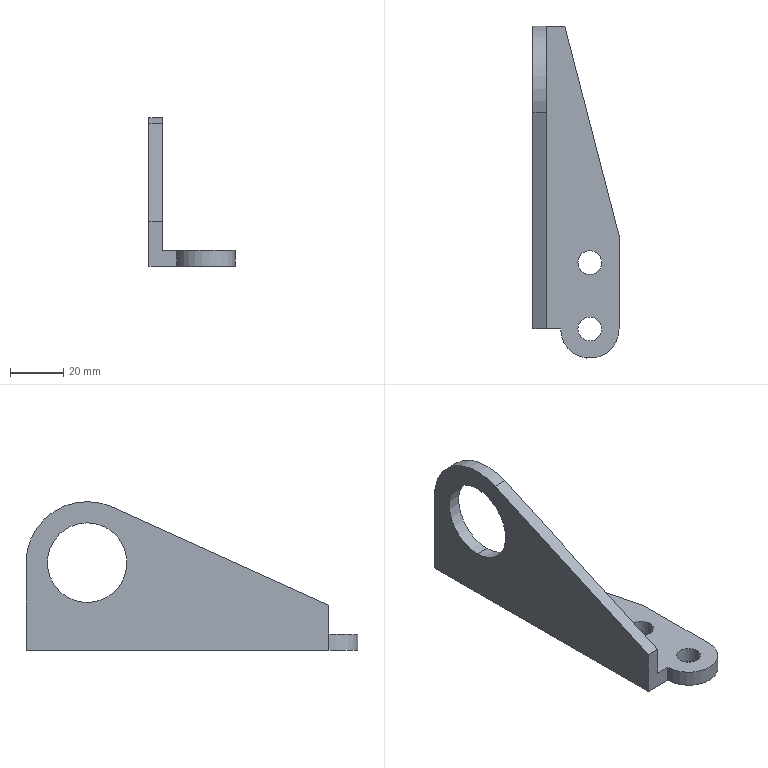Part | SolidWorks | features BaseBody 1 | 1 solid | 17 faces | box 32.409 x 125 x 56 mm | volume 33709 mm3 | plane 9 | cylinder 8 | commonest cylinder face diameters 9 x4 30 x2 22 x1 46 x1
STEP:
#1=CARTESIAN_POINT('',(-12.659,449.35,-210.5));
#2=VERTEX_POINT('',#1);
#3=CARTESIAN_POINT('',(-12.659,449.35,-180.5));
#4=VERTEX_POINT('',#3);
#5=CARTESIAN_POINT('',(-12.659,449.35,-195.5));
#6=DIRECTION('',(-1.,0.,0.));
#7=DIRECTION('',(0.,0.,-1.));
#8=AXIS2_PLACEMENT_3D('',#5,#6,#7);
#9=CIRCLE('',#8,15.);
#10=EDGE_CURVE('',#2,#4,#9,.T.);
#11=ORIENTED_EDGE('',*,*,#10,.T.);
#12=CARTESIAN_POINT('',(-7.659,449.35,-180.5));
#13=VERTEX_POINT('',#12);
#14=CARTESIAN_POINT('',(-12.659,449.35,-180.5));
#15=DIRECTION('',(1.,0.,0.));
#16=VECTOR('',#15,1000.);
#17=LINE('',#14,#16);
#18=EDGE_CURVE('',#4,#13,#17,.T.);
#19=ORIENTED_EDGE('',*,*,#18,.T.);
#20=CARTESIAN_POINT('',(-7.659,449.35,-210.5));
#21=VERTEX_POINT('',#20);
#22=CARTESIAN_POINT('',(-7.659,449.35,-195.5));
#23=DIRECTION('',(-1.,0.,0.));
#24=DIRECTION('',(0.,0.,-1.));
#25=AXIS2_PLACEMENT_3D('',#22,#23,#24);
#26=CIRCLE('',#25,15.);
#27=EDGE_CURVE('',#21,#13,#26,.T.);
#28=ORIENTED_EDGE('',*,*,#27,.F.);
#29=CARTESIAN_POINT('',(-12.659,449.35,-210.5));
#30=DIRECTION('',(1.,0.,0.));
#31=VECTOR('',#30,1000.);
#32=LINE('',#29,#31);
#33=EDGE_CURVE('',#2,#21,#32,.T.);
#34=ORIENTED_EDGE('',*,*,#33,.F.);
#35=EDGE_LOOP('',(#11,#19,#28,#34));
#36=FACE_OUTER_BOUND('',#35,.T.);
#37=CARTESIAN_POINT('',(-12.659,449.35,-195.5));
#38=DIRECTION('',(1.,0.,0.));
#39=DIRECTION('',(0.,0.,-1.));
#40=AXIS2_PLACEMENT_3D('',#37,#38,#39);
#41=CYLINDRICAL_SURFACE('',#40,15.);
#42=ADVANCED_FACE('',(#36),#41,.F.);
#43=CARTESIAN_POINT('',(13.25,358.35,-222.5));
#44=VERTEX_POINT('',#43);
#45=CARTESIAN_POINT('',(4.25,358.35,-222.5));
#46=VERTEX_POINT('',#45);
#47=CARTESIAN_POINT('',(8.75,358.35,-222.5));
#48=DIRECTION('',(0.,0.,-1.));
#49=DIRECTION('',(-1.,0.,0.));
#50=AXIS2_PLACEMENT_3D('',#47,#48,#49);
#51=CIRCLE('',#50,4.5);
#52=EDGE_CURVE('',#44,#46,#51,.T.);
#53=ORIENTED_EDGE('',*,*,#52,.F.);
#54=CARTESIAN_POINT('',(13.25,358.35,-228.5));
#55=VERTEX_POINT('',#54);
#56=CARTESIAN_POINT('',(13.25,358.35,-222.5));
#57=DIRECTION('',(0.,0.,-1.));
#58=VECTOR('',#57,1000.);
#59=LINE('',#56,#58);
#60=EDGE_CURVE('',#44,#55,#59,.T.);
#61=ORIENTED_EDGE('',*,*,#60,.T.);
#62=CARTESIAN_POINT('',(4.25,358.35,-228.5));
#63=VERTEX_POINT('',#62);
#64=CARTESIAN_POINT('',(8.75,358.35,-228.5));
#65=DIRECTION('',(0.,0.,-1.));
#66=DIRECTION('',(-1.,0.,0.));
#67=AXIS2_PLACEMENT_3D('',#64,#65,#66);
#68=CIRCLE('',#67,4.5);
#69=EDGE_CURVE('',#55,#63,#68,.T.);
#70=ORIENTED_EDGE('',*,*,#69,.T.);
#71=CARTESIAN_POINT('',(4.25,358.35,-222.5));
#72=DIRECTION('',(0.,0.,-1.));
#73=VECTOR('',#72,1000.);
#74=LINE('',#71,#73);
#75=EDGE_CURVE('',#46,#63,#74,.T.);
#76=ORIENTED_EDGE('',*,*,#75,.F.);
#77=EDGE_LOOP('',(#53,#61,#70,#76));
#78=FACE_OUTER_BOUND('',#77,.T.);
#79=CARTESIAN_POINT('',(8.75,358.35,-222.5));
#80=DIRECTION('',(0.,0.,-1.));
#81=DIRECTION('',(-1.,0.,0.));
#82=AXIS2_PLACEMENT_3D('',#79,#80,#81);
#83=CYLINDRICAL_SURFACE('',#82,4.5);
#84=ADVANCED_FACE('',(#78),#83,.F.);
#85=CARTESIAN_POINT('',(13.25,383.35,-222.5));
#86=VERTEX_POINT('',#85);
#87=CARTESIAN_POINT('',(4.25,383.35,-222.5));
#88=VERTEX_POINT('',#87);
#89=CARTESIAN_POINT('',(8.75,383.35,-222.5));
#90=DIRECTION('',(0.,0.,-1.));
#91=DIRECTION('',(-1.,0.,0.));
#92=AXIS2_PLACEMENT_3D('',#89,#90,#91);
#93=CIRCLE('',#92,4.5);
#94=EDGE_CURVE('',#86,#88,#93,.T.);
#95=ORIENTED_EDGE('',*,*,#94,.F.);
#96=CARTESIAN_POINT('',(13.25,383.35,-228.5));
#97=VERTEX_POINT('',#96);
#98=CARTESIAN_POINT('',(13.25,383.35,-222.5));
#99=DIRECTION('',(0.,0.,-1.));
#100=VECTOR('',#99,1000.);
#101=LINE('',#98,#100);
#102=EDGE_CURVE('',#86,#97,#101,.T.);
#103=ORIENTED_EDGE('',*,*,#102,.T.);
#104=CARTESIAN_POINT('',(4.25,383.35,-228.5));
#105=VERTEX_POINT('',#104);
#106=CARTESIAN_POINT('',(8.75,383.35,-228.5));
#107=DIRECTION('',(0.,0.,-1.));
#108=DIRECTION('',(-1.,0.,0.));
#109=AXIS2_PLACEMENT_3D('',#106,#107,#108);
#110=CIRCLE('',#109,4.5);
#111=EDGE_CURVE('',#97,#105,#110,.T.);
#112=ORIENTED_EDGE('',*,*,#111,.T.);
#113=CARTESIAN_POINT('',(4.25,383.35,-222.5));
#114=DIRECTION('',(0.,0.,-1.));
#115=VECTOR('',#114,1000.);
#116=LINE('',#113,#115);
#117=EDGE_CURVE('',#88,#105,#116,.T.);
#118=ORIENTED_EDGE('',*,*,#117,.F.);
#119=EDGE_LOOP('',(#95,#103,#112,#118));
#120=FACE_OUTER_BOUND('',#119,.T.);
#121=CARTESIAN_POINT('',(8.75,383.35,-222.5));
#122=DIRECTION('',(0.,0.,-1.));
#123=DIRECTION('',(-1.,0.,0.));
#124=AXIS2_PLACEMENT_3D('',#121,#122,#123);
#125=CYLINDRICAL_SURFACE('',#124,4.5);
#126=ADVANCED_FACE('',(#120),#125,.F.);
#127=ORIENTED_EDGE('',*,*,#10,.F.);
#128=CARTESIAN_POINT('',(-12.659,449.35,-195.5));
#129=DIRECTION('',(-1.,0.,0.));
#130=DIRECTION('',(0.,0.,-1.));
#131=AXIS2_PLACEMENT_3D('',#128,#129,#130);
#132=CIRCLE('',#131,15.);
#133=EDGE_CURVE('',#4,#2,#132,.T.);
#134=ORIENTED_EDGE('',*,*,#133,.F.);
#135=EDGE_LOOP('',(#127,#134));
#136=FACE_BOUND('',#135,.T.);
#137=CARTESIAN_POINT('',(-12.659,358.35,-211.5));
#138=VERTEX_POINT('',#137);
#139=CARTESIAN_POINT('',(-12.659,358.35,-228.5));
#140=VERTEX_POINT('',#139);
#141=CARTESIAN_POINT('',(-12.659,358.35,-200.491));
#142=DIRECTION('',(0.,0.,-1.));
#143=VECTOR('',#142,1000.);
#144=LINE('',#141,#143);
#145=EDGE_CURVE('',#138,#140,#144,.T.);
#146=ORIENTED_EDGE('',*,*,#145,.F.);
#147=CARTESIAN_POINT('',(-12.659,439.854,-174.552));
#148=VERTEX_POINT('',#147);
#149=CARTESIAN_POINT('',(-12.659,439.854,-174.552));
#150=DIRECTION('',(0.,-0.9108,-0.4129));
#151=VECTOR('',#150,1000.);
#152=LINE('',#149,#151);
#153=EDGE_CURVE('',#148,#138,#152,.T.);
#154=ORIENTED_EDGE('',*,*,#153,.F.);
#155=CARTESIAN_POINT('',(-12.659,472.35,-195.5));
#156=VERTEX_POINT('',#155);
#157=CARTESIAN_POINT('',(-12.659,449.35,-195.5));
#158=DIRECTION('',(1.,0.,0.));
#159=DIRECTION('',(0.,0.,-1.));
#160=AXIS2_PLACEMENT_3D('',#157,#158,#159);
#161=CIRCLE('',#160,23.);
#162=EDGE_CURVE('',#156,#148,#161,.T.);
#163=ORIENTED_EDGE('',*,*,#162,.F.);
#164=CARTESIAN_POINT('',(-12.659,472.35,-228.5));
#165=VERTEX_POINT('',#164);
#166=CARTESIAN_POINT('',(-12.659,472.35,-200.491));
#167=DIRECTION('',(0.,0.,1.));
#168=VECTOR('',#167,1000.);
#169=LINE('',#166,#168);
#170=EDGE_CURVE('',#165,#156,#169,.T.);
#171=ORIENTED_EDGE('',*,*,#170,.F.);
#172=CARTESIAN_POINT('',(-12.659,415.35,-228.5));
#173=DIRECTION('',(0.,1.,0.));
#174=VECTOR('',#173,1000.);
#175=LINE('',#172,#174);
#176=EDGE_CURVE('',#140,#165,#175,.T.);
#177=ORIENTED_EDGE('',*,*,#176,.F.);
#178=EDGE_LOOP('',(#146,#154,#163,#171,#177));
#179=FACE_OUTER_BOUND('',#178,.T.);
#180=CARTESIAN_POINT('',(-12.659,415.35,-200.491));
#181=DIRECTION('',(1.,0.,0.));
#182=DIRECTION('',(0.,0.,-1.));
#183=AXIS2_PLACEMENT_3D('',#180,#181,#182);
#184=PLANE('',#183);
#185=ADVANCED_FACE('',(#136,#179),#184,.F.);
#186=ORIENTED_EDGE('',*,*,#18,.F.);
#187=ORIENTED_EDGE('',*,*,#133,.T.);
#188=ORIENTED_EDGE('',*,*,#33,.T.);
#189=CARTESIAN_POINT('',(-7.659,449.35,-195.5));
#190=DIRECTION('',(-1.,0.,0.));
#191=DIRECTION('',(0.,0.,-1.));
#192=AXIS2_PLACEMENT_3D('',#189,#190,#191);
#193=CIRCLE('',#192,15.);
#194=EDGE_CURVE('',#13,#21,#193,.T.);
#195=ORIENTED_EDGE('',*,*,#194,.F.);
#196=EDGE_LOOP('',(#186,#187,#188,#195));
#197=FACE_OUTER_BOUND('',#196,.T.);
#198=CARTESIAN_POINT('',(-12.659,449.35,-195.5));
#199=DIRECTION('',(1.,0.,0.));
#200=DIRECTION('',(0.,0.,-1.));
#201=AXIS2_PLACEMENT_3D('',#198,#199,#200);
#202=CYLINDRICAL_SURFACE('',#201,15.);
#203=ADVANCED_FACE('',(#197),#202,.F.);
#204=CARTESIAN_POINT('',(8.75,358.35,-228.5));
#205=DIRECTION('',(0.,0.,-1.));
#206=DIRECTION('',(-1.,0.,0.));
#207=AXIS2_PLACEMENT_3D('',#204,#205,#206);
#208=CIRCLE('',#207,4.5);
#209=EDGE_CURVE('',#63,#55,#208,.T.);
#210=ORIENTED_EDGE('',*,*,#209,.F.);
#211=ORIENTED_EDGE('',*,*,#69,.F.);
#212=EDGE_LOOP('',(#210,#211));
#213=FACE_BOUND('',#212,.T.);
#214=CARTESIAN_POINT('',(8.75,383.35,-228.5));
#215=DIRECTION('',(0.,0.,-1.));
#216=DIRECTION('',(-1.,0.,0.));
#217=AXIS2_PLACEMENT_3D('',#214,#215,#216);
#218=CIRCLE('',#217,4.5);
#219=EDGE_CURVE('',#105,#97,#218,.T.);
#220=ORIENTED_EDGE('',*,*,#219,.F.);
#221=ORIENTED_EDGE('',*,*,#111,.F.);
#222=EDGE_LOOP('',(#220,#221));
#223=FACE_BOUND('',#222,.T.);
#224=ORIENTED_EDGE('',*,*,#176,.T.);
#225=CARTESIAN_POINT('',(-0.6587,472.35,-228.5));
#226=VERTEX_POINT('',#225);
#227=CARTESIAN_POINT('',(3.546,472.35,-228.5));
#228=DIRECTION('',(-1.,0.,0.));
#229=VECTOR('',#228,1000.);
#230=LINE('',#227,#229);
#231=EDGE_CURVE('',#226,#165,#230,.T.);
#232=ORIENTED_EDGE('',*,*,#231,.F.);
#233=CARTESIAN_POINT('',(19.75,393.35,-228.5));
#234=VERTEX_POINT('',#233);
#235=CARTESIAN_POINT('',(19.75,393.35,-228.5));
#236=DIRECTION('',(-0.2501,0.9682,0.));
#237=VECTOR('',#236,1000.);
#238=LINE('',#235,#237);
#239=EDGE_CURVE('',#234,#226,#238,.T.);
#240=ORIENTED_EDGE('',*,*,#239,.F.);
#241=CARTESIAN_POINT('',(19.75,358.35,-228.5));
#242=VERTEX_POINT('',#241);
#243=CARTESIAN_POINT('',(19.75,409.85,-228.5));
#244=DIRECTION('',(0.,1.,0.));
#245=VECTOR('',#244,1000.);
#246=LINE('',#243,#245);
#247=EDGE_CURVE('',#242,#234,#246,.T.);
#248=ORIENTED_EDGE('',*,*,#247,.F.);
#249=CARTESIAN_POINT('',(-2.25,358.35,-228.5));
#250=VERTEX_POINT('',#249);
#251=CARTESIAN_POINT('',(8.75,358.35,-228.5));
#252=DIRECTION('',(0.,0.,1.));
#253=DIRECTION('',(-1.,0.,0.));
#254=AXIS2_PLACEMENT_3D('',#251,#252,#253);
#255=CIRCLE('',#254,11.);
#256=EDGE_CURVE('',#250,#242,#255,.T.);
#257=ORIENTED_EDGE('',*,*,#256,.F.);
#258=CARTESIAN_POINT('',(3.546,358.35,-228.5));
#259=DIRECTION('',(1.,0.,0.));
#260=VECTOR('',#259,1000.);
#261=LINE('',#258,#260);
#262=EDGE_CURVE('',#140,#250,#261,.T.);
#263=ORIENTED_EDGE('',*,*,#262,.F.);
#264=EDGE_LOOP('',(#224,#232,#240,#248,#257,#263));
#265=FACE_OUTER_BOUND('',#264,.T.);
#266=CARTESIAN_POINT('',(3.546,409.85,-228.5));
#267=DIRECTION('',(0.,0.,1.));
#268=DIRECTION('',(1.,0.,0.));
#269=AXIS2_PLACEMENT_3D('',#266,#267,#268);
#270=PLANE('',#269);
#271=ADVANCED_FACE('',(#213,#223,#265),#270,.F.);
#272=CARTESIAN_POINT('',(-7.659,358.35,-211.5));
#273=VERTEX_POINT('',#272);
#274=CARTESIAN_POINT('',(-7.454,358.35,-211.5));
#275=DIRECTION('',(1.,0.,0.));
#276=VECTOR('',#275,1000.);
#277=LINE('',#274,#276);
#278=EDGE_CURVE('',#138,#273,#277,.T.);
#279=ORIENTED_EDGE('',*,*,#278,.F.);
#280=ORIENTED_EDGE('',*,*,#145,.T.);
#281=ORIENTED_EDGE('',*,*,#262,.T.);
#282=CARTESIAN_POINT('',(-2.25,358.35,-222.5));
#283=VERTEX_POINT('',#282);
#284=CARTESIAN_POINT('',(-2.25,358.35,-220.));
#285=DIRECTION('',(0.,0.,-1.));
#286=VECTOR('',#285,1000.);
#287=LINE('',#284,#286);
#288=EDGE_CURVE('',#283,#250,#287,.T.);
#289=ORIENTED_EDGE('',*,*,#288,.F.);
#290=CARTESIAN_POINT('',(-7.659,358.35,-222.5));
#291=VERTEX_POINT('',#290);
#292=CARTESIAN_POINT('',(-7.454,358.35,-222.5));
#293=DIRECTION('',(1.,0.,0.));
#294=VECTOR('',#293,1000.);
#295=LINE('',#292,#294);
#296=EDGE_CURVE('',#291,#283,#295,.T.);
#297=ORIENTED_EDGE('',*,*,#296,.F.);
#298=CARTESIAN_POINT('',(-7.659,358.35,-220.));
#299=DIRECTION('',(0.,0.,-1.));
#300=VECTOR('',#299,1000.);
#301=LINE('',#298,#300);
#302=EDGE_CURVE('',#273,#291,#301,.T.);
#303=ORIENTED_EDGE('',*,*,#302,.F.);
#304=EDGE_LOOP('',(#279,#280,#281,#289,#297,#303));
#305=FACE_OUTER_BOUND('',#304,.T.);
#306=CARTESIAN_POINT('',(-7.454,358.35,-220.));
#307=DIRECTION('',(0.,1.,0.));
#308=DIRECTION('',(0.,0.,1.));
#309=AXIS2_PLACEMENT_3D('',#306,#307,#308);
#310=PLANE('',#309);
#311=ADVANCED_FACE('',(#305),#310,.F.);
#312=ORIENTED_EDGE('',*,*,#278,.T.);
#313=CARTESIAN_POINT('',(-7.659,439.854,-174.552));
#314=VERTEX_POINT('',#313);
#315=CARTESIAN_POINT('',(-7.659,399.102,-193.026));
#316=DIRECTION('',(0.,0.9108,0.4129));
#317=VECTOR('',#316,1000.);
#318=LINE('',#315,#317);
#319=EDGE_CURVE('',#273,#314,#318,.T.);
#320=ORIENTED_EDGE('',*,*,#319,.T.);
#321=CARTESIAN_POINT('',(-10.159,439.854,-174.552));
#322=DIRECTION('',(-1.,0.,0.));
#323=VECTOR('',#322,1000.);
#324=LINE('',#321,#323);
#325=EDGE_CURVE('',#314,#148,#324,.T.);
#326=ORIENTED_EDGE('',*,*,#325,.T.);
#327=ORIENTED_EDGE('',*,*,#153,.T.);
#328=EDGE_LOOP('',(#312,#320,#326,#327));
#329=FACE_OUTER_BOUND('',#328,.T.);
#330=CARTESIAN_POINT('',(-10.159,399.102,-193.026));
#331=DIRECTION('',(0.,-0.4129,0.9108));
#332=DIRECTION('',(0.,-0.9108,-0.4129));
#333=AXIS2_PLACEMENT_3D('',#330,#331,#332);
#334=PLANE('',#333);
#335=ADVANCED_FACE('',(#329),#334,.T.);
#336=ORIENTED_EDGE('',*,*,#162,.T.);
#337=ORIENTED_EDGE('',*,*,#325,.F.);
#338=CARTESIAN_POINT('',(-7.659,472.35,-195.5));
#339=VERTEX_POINT('',#338);
#340=CARTESIAN_POINT('',(-7.659,449.35,-195.5));
#341=DIRECTION('',(-1.,0.,0.));
#342=DIRECTION('',(0.,0.,-1.));
#343=AXIS2_PLACEMENT_3D('',#340,#341,#342);
#344=CIRCLE('',#343,23.);
#345=EDGE_CURVE('',#314,#339,#344,.T.);
#346=ORIENTED_EDGE('',*,*,#345,.T.);
#347=CARTESIAN_POINT('',(-12.659,472.35,-195.5));
#348=DIRECTION('',(-1.,0.,0.));
#349=VECTOR('',#348,1000.);
#350=LINE('',#347,#349);
#351=EDGE_CURVE('',#339,#156,#350,.T.);
#352=ORIENTED_EDGE('',*,*,#351,.T.);
#353=EDGE_LOOP('',(#336,#337,#346,#352));
#354=FACE_OUTER_BOUND('',#353,.T.);
#355=CARTESIAN_POINT('',(-12.659,449.35,-195.5));
#356=DIRECTION('',(1.,0.,0.));
#357=DIRECTION('',(0.,0.,-1.));
#358=AXIS2_PLACEMENT_3D('',#355,#356,#357);
#359=CYLINDRICAL_SURFACE('',#358,23.);
#360=ADVANCED_FACE('',(#354),#359,.T.);
#361=ORIENTED_EDGE('',*,*,#231,.T.);
#362=ORIENTED_EDGE('',*,*,#170,.T.);
#363=ORIENTED_EDGE('',*,*,#351,.F.);
#364=CARTESIAN_POINT('',(-7.659,472.35,-222.5));
#365=VERTEX_POINT('',#364);
#366=CARTESIAN_POINT('',(-7.659,472.35,-212.));
#367=DIRECTION('',(0.,0.,-1.));
#368=VECTOR('',#367,1000.);
#369=LINE('',#366,#368);
#370=EDGE_CURVE('',#339,#365,#369,.T.);
#371=ORIENTED_EDGE('',*,*,#370,.T.);
#372=CARTESIAN_POINT('',(-0.6587,472.35,-222.5));
#373=VERTEX_POINT('',#372);
#374=CARTESIAN_POINT('',(-6.659,472.35,-222.5));
#375=DIRECTION('',(1.,0.,0.));
#376=VECTOR('',#375,1000.);
#377=LINE('',#374,#376);
#378=EDGE_CURVE('',#365,#373,#377,.T.);
#379=ORIENTED_EDGE('',*,*,#378,.T.);
#380=CARTESIAN_POINT('',(-0.6587,472.35,-212.));
#381=DIRECTION('',(0.,0.,-1.));
#382=VECTOR('',#381,1000.);
#383=LINE('',#380,#382);
#384=EDGE_CURVE('',#373,#226,#383,.T.);
#385=ORIENTED_EDGE('',*,*,#384,.T.);
#386=EDGE_LOOP('',(#361,#362,#363,#371,#379,#385));
#387=FACE_OUTER_BOUND('',#386,.T.);
#388=CARTESIAN_POINT('',(-6.659,472.35,-212.));
#389=DIRECTION('',(0.,1.,0.));
#390=DIRECTION('',(0.,0.,1.));
#391=AXIS2_PLACEMENT_3D('',#388,#389,#390);
#392=PLANE('',#391);
#393=ADVANCED_FACE('',(#387),#392,.T.);
#394=ORIENTED_EDGE('',*,*,#27,.T.);
#395=ORIENTED_EDGE('',*,*,#194,.T.);
#396=EDGE_LOOP('',(#394,#395));
#397=FACE_BOUND('',#396,.T.);
#398=ORIENTED_EDGE('',*,*,#302,.T.);
#399=CARTESIAN_POINT('',(-7.659,415.35,-222.5));
#400=DIRECTION('',(0.,1.,0.));
#401=VECTOR('',#400,1000.);
#402=LINE('',#399,#401);
#403=EDGE_CURVE('',#291,#365,#402,.T.);
#404=ORIENTED_EDGE('',*,*,#403,.T.);
#405=ORIENTED_EDGE('',*,*,#370,.F.);
#406=ORIENTED_EDGE('',*,*,#345,.F.);
#407=ORIENTED_EDGE('',*,*,#319,.F.);
#408=EDGE_LOOP('',(#398,#404,#405,#406,#407));
#409=FACE_OUTER_BOUND('',#408,.T.);
#410=CARTESIAN_POINT('',(-7.659,415.35,-197.491));
#411=DIRECTION('',(1.,0.,0.));
#412=DIRECTION('',(0.,0.,-1.));
#413=AXIS2_PLACEMENT_3D('',#410,#411,#412);
#414=PLANE('',#413);
#415=ADVANCED_FACE('',(#397,#409),#414,.T.);
#416=ORIENTED_EDGE('',*,*,#60,.F.);
#417=CARTESIAN_POINT('',(8.75,358.35,-222.5));
#418=DIRECTION('',(0.,0.,-1.));
#419=DIRECTION('',(-1.,0.,0.));
#420=AXIS2_PLACEMENT_3D('',#417,#418,#419);
#421=CIRCLE('',#420,4.5);
#422=EDGE_CURVE('',#46,#44,#421,.T.);
#423=ORIENTED_EDGE('',*,*,#422,.F.);
#424=ORIENTED_EDGE('',*,*,#75,.T.);
#425=ORIENTED_EDGE('',*,*,#209,.T.);
#426=EDGE_LOOP('',(#416,#423,#424,#425));
#427=FACE_OUTER_BOUND('',#426,.T.);
#428=CARTESIAN_POINT('',(8.75,358.35,-222.5));
#429=DIRECTION('',(0.,0.,-1.));
#430=DIRECTION('',(-1.,0.,0.));
#431=AXIS2_PLACEMENT_3D('',#428,#429,#430);
#432=CYLINDRICAL_SURFACE('',#431,4.5);
#433=ADVANCED_FACE('',(#427),#432,.F.);
#434=ORIENTED_EDGE('',*,*,#102,.F.);
#435=CARTESIAN_POINT('',(8.75,383.35,-222.5));
#436=DIRECTION('',(0.,0.,-1.));
#437=DIRECTION('',(-1.,0.,0.));
#438=AXIS2_PLACEMENT_3D('',#435,#436,#437);
#439=CIRCLE('',#438,4.5);
#440=EDGE_CURVE('',#88,#86,#439,.T.);
#441=ORIENTED_EDGE('',*,*,#440,.F.);
#442=ORIENTED_EDGE('',*,*,#117,.T.);
#443=ORIENTED_EDGE('',*,*,#219,.T.);
#444=EDGE_LOOP('',(#434,#441,#442,#443));
#445=FACE_OUTER_BOUND('',#444,.T.);
#446=CARTESIAN_POINT('',(8.75,383.35,-222.5));
#447=DIRECTION('',(0.,0.,-1.));
#448=DIRECTION('',(-1.,0.,0.));
#449=AXIS2_PLACEMENT_3D('',#446,#447,#448);
#450=CYLINDRICAL_SURFACE('',#449,4.5);
#451=ADVANCED_FACE('',(#445),#450,.F.);
#452=CARTESIAN_POINT('',(19.75,393.35,-222.5));
#453=VERTEX_POINT('',#452);
#454=CARTESIAN_POINT('',(19.75,393.35,-225.5));
#455=DIRECTION('',(0.,0.,-1.));
#456=VECTOR('',#455,1000.);
#457=LINE('',#454,#456);
#458=EDGE_CURVE('',#453,#234,#457,.T.);
#459=ORIENTED_EDGE('',*,*,#458,.T.);
#460=ORIENTED_EDGE('',*,*,#239,.T.);
#461=ORIENTED_EDGE('',*,*,#384,.F.);
#462=CARTESIAN_POINT('',(9.546,432.85,-222.5));
#463=DIRECTION('',(0.2501,-0.9682,0.));
#464=VECTOR('',#463,1000.);
#465=LINE('',#462,#464);
#466=EDGE_CURVE('',#373,#453,#465,.T.);
#467=ORIENTED_EDGE('',*,*,#466,.T.);
#468=EDGE_LOOP('',(#459,#460,#461,#467));
#469=FACE_OUTER_BOUND('',#468,.T.);
#470=CARTESIAN_POINT('',(9.546,432.85,-225.5));
#471=DIRECTION('',(0.9682,0.2501,0.));
#472=DIRECTION('',(-0.2501,0.9682,0.));
#473=AXIS2_PLACEMENT_3D('',#470,#471,#472);
#474=PLANE('',#473);
#475=ADVANCED_FACE('',(#469),#474,.T.);
#476=CARTESIAN_POINT('',(19.75,358.35,-222.5));
#477=VERTEX_POINT('',#476);
#478=CARTESIAN_POINT('',(19.75,358.35,-225.5));
#479=DIRECTION('',(0.,0.,-1.));
#480=VECTOR('',#479,1000.);
#481=LINE('',#478,#480);
#482=EDGE_CURVE('',#477,#242,#481,.T.);
#483=ORIENTED_EDGE('',*,*,#482,.T.);
#484=ORIENTED_EDGE('',*,*,#247,.T.);
#485=ORIENTED_EDGE('',*,*,#458,.F.);
#486=CARTESIAN_POINT('',(19.75,375.85,-222.5));
#487=DIRECTION('',(0.,-1.,0.));
#488=VECTOR('',#487,1000.);
#489=LINE('',#486,#488);
#490=EDGE_CURVE('',#453,#477,#489,.T.);
#491=ORIENTED_EDGE('',*,*,#490,.T.);
#492=EDGE_LOOP('',(#483,#484,#485,#491));
#493=FACE_OUTER_BOUND('',#492,.T.);
#494=CARTESIAN_POINT('',(19.75,375.85,-225.5));
#495=DIRECTION('',(1.,0.,0.));
#496=DIRECTION('',(0.,0.,-1.));
#497=AXIS2_PLACEMENT_3D('',#494,#495,#496);
#498=PLANE('',#497);
#499=ADVANCED_FACE('',(#493),#498,.T.);
#500=CARTESIAN_POINT('',(8.75,358.35,-222.5));
#501=DIRECTION('',(0.,0.,-1.));
#502=DIRECTION('',(-1.,0.,0.));
#503=AXIS2_PLACEMENT_3D('',#500,#501,#502);
#504=CIRCLE('',#503,11.);
#505=EDGE_CURVE('',#477,#283,#504,.T.);
#506=ORIENTED_EDGE('',*,*,#505,.T.);
#507=ORIENTED_EDGE('',*,*,#288,.T.);
#508=ORIENTED_EDGE('',*,*,#256,.T.);
#509=ORIENTED_EDGE('',*,*,#482,.F.);
#510=EDGE_LOOP('',(#506,#507,#508,#509));
#511=FACE_OUTER_BOUND('',#510,.T.);
#512=CARTESIAN_POINT('',(8.75,358.35,-222.5));
#513=DIRECTION('',(0.,0.,-1.));
#514=DIRECTION('',(-1.,0.,0.));
#515=AXIS2_PLACEMENT_3D('',#512,#513,#514);
#516=CYLINDRICAL_SURFACE('',#515,11.);
#517=ADVANCED_FACE('',(#511),#516,.T.);
#518=ORIENTED_EDGE('',*,*,#422,.T.);
#519=ORIENTED_EDGE('',*,*,#52,.T.);
#520=EDGE_LOOP('',(#518,#519));
#521=FACE_BOUND('',#520,.T.);
#522=ORIENTED_EDGE('',*,*,#440,.T.);
#523=ORIENTED_EDGE('',*,*,#94,.T.);
#524=EDGE_LOOP('',(#522,#523));
#525=FACE_BOUND('',#524,.T.);
#526=ORIENTED_EDGE('',*,*,#403,.F.);
#527=ORIENTED_EDGE('',*,*,#296,.T.);
#528=ORIENTED_EDGE('',*,*,#505,.F.);
#529=ORIENTED_EDGE('',*,*,#490,.F.);
#530=ORIENTED_EDGE('',*,*,#466,.F.);
#531=ORIENTED_EDGE('',*,*,#378,.F.);
#532=EDGE_LOOP('',(#526,#527,#528,#529,#530,#531));
#533=FACE_OUTER_BOUND('',#532,.T.);
#534=CARTESIAN_POINT('',(6.046,409.85,-222.5));
#535=DIRECTION('',(0.,0.,1.));
#536=DIRECTION('',(1.,0.,0.));
#537=AXIS2_PLACEMENT_3D('',#534,#535,#536);
#538=PLANE('',#537);
#539=ADVANCED_FACE('',(#521,#525,#533),#538,.T.);
#540=CLOSED_SHELL('',(#42,#84,#126,#185,#203,#271,#311,#335,#360,#393,#415,#433,#451,#475,#499,#517,#539));
#541=MANIFOLD_SOLID_BREP('',#540);
#542=CARTESIAN_POINT('',(0.,0.,0.));
#543=DIRECTION('',(0.,0.,1.));
#544=DIRECTION('',(1.,0.,0.));
#545=AXIS2_PLACEMENT_3D('',#542,#543,#544);
#546=(LENGTH_UNIT()NAMED_UNIT(*)SI_UNIT(.MILLI.,.METRE.));
#547=UNCERTAINTY_MEASURE_WITH_UNIT(LENGTH_MEASURE(0.00001),#546,'','');
#548=(NAMED_UNIT(*)PLANE_ANGLE_UNIT()SI_UNIT($,.RADIAN.));
#549=(NAMED_UNIT(*)SI_UNIT($,.STERADIAN.)SOLID_ANGLE_UNIT());
#550=(GEOMETRIC_REPRESENTATION_CONTEXT(3)GLOBAL_UNCERTAINTY_ASSIGNED_CONTEXT((#547))GLOBAL_UNIT_ASSIGNED_CONTEXT((#546,#548,#549))REPRESENTATION_CONTEXT('',''));
#551=ADVANCED_BREP_SHAPE_REPRESENTATION('',(#541,#545),#550);